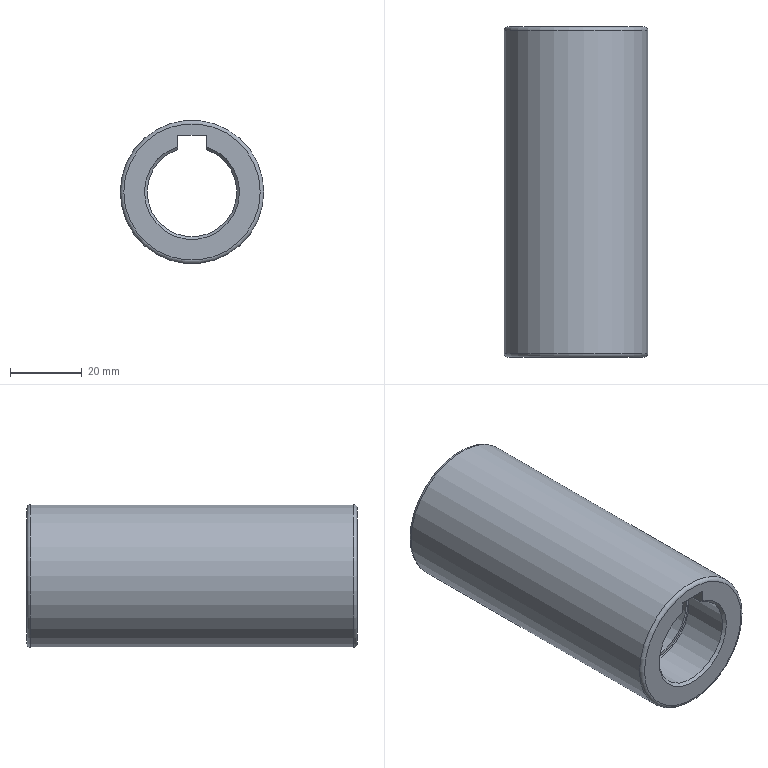Part | STEP file | 冲床-300配套压波_id1126_x_t | 1 solid | 23 faces | box 40 x 92 x 40 mm | volume 67089 mm3 | plane 11 | cylinder 8 | cone 2 | torus 2 | commonest cylinder face diameters 25 x4 26.5 x2 25.5 x1 40 x1
STEP:
#1=CARTESIAN_POINT('',(1388.,32.,91.926));
#2=VERTEX_POINT('',#1);
#3=CARTESIAN_POINT('',(1388.,45.25,91.926));
#4=VERTEX_POINT('',#3);
#5=CARTESIAN_POINT('',(1388.,-46.,91.926));
#6=DIRECTION('',(0.,1.,0.));
#7=VECTOR('',#6,1.);
#8=LINE('',#5,#7);
#9=EDGE_CURVE('',#2,#4,#8,.T.);
#10=ORIENTED_EDGE('',*,*,#9,.T.);
#11=CARTESIAN_POINT('',(1388.,46.,92.715));
#12=VERTEX_POINT('',#11);
#13=CARTESIAN_POINT('',(1388.,45.25,91.926));
#14=CARTESIAN_POINT('',(1388.,45.5,92.19));
#15=CARTESIAN_POINT('',(1388.,45.75,92.453));
#16=CARTESIAN_POINT('',(1388.,46.,92.715));
#17=B_SPLINE_CURVE_WITH_KNOTS('',3,(#13,#14,#15,#16),.UNSPECIFIED.,.F.,.F.,(4,4),(0.,1.),.UNSPECIFIED.);
#18=EDGE_CURVE('',#4,#12,#17,.T.);
#19=ORIENTED_EDGE('',*,*,#18,.T.);
#20=CARTESIAN_POINT('',(1388.,46.,95.883));
#21=VERTEX_POINT('',#20);
#22=CARTESIAN_POINT('',(1388.,46.,95.883));
#23=DIRECTION('',(0.,0.,-1.));
#24=VECTOR('',#23,1.);
#25=LINE('',#22,#24);
#26=EDGE_CURVE('',#21,#12,#25,.T.);
#27=ORIENTED_EDGE('',*,*,#26,.F.);
#28=CARTESIAN_POINT('',(1388.,-46.,95.883));
#29=VERTEX_POINT('',#28);
#30=CARTESIAN_POINT('',(1388.,-46.,95.883));
#31=DIRECTION('',(0.,1.,0.));
#32=VECTOR('',#31,1.);
#33=LINE('',#30,#32);
#34=EDGE_CURVE('',#29,#21,#33,.T.);
#35=ORIENTED_EDGE('',*,*,#34,.F.);
#36=CARTESIAN_POINT('',(1388.,-46.,92.715));
#37=VERTEX_POINT('',#36);
#38=CARTESIAN_POINT('',(1388.,-46.,95.883));
#39=DIRECTION('',(0.,0.,-1.));
#40=VECTOR('',#39,1.);
#41=LINE('',#38,#40);
#42=EDGE_CURVE('',#29,#37,#41,.T.);
#43=ORIENTED_EDGE('',*,*,#42,.T.);
#44=CARTESIAN_POINT('',(1388.,-45.25,91.926));
#45=VERTEX_POINT('',#44);
#46=CARTESIAN_POINT('',(1388.,-46.,92.715));
#47=CARTESIAN_POINT('',(1388.,-45.75,92.453));
#48=CARTESIAN_POINT('',(1388.,-45.5,92.19));
#49=CARTESIAN_POINT('',(1388.,-45.25,91.926));
#50=B_SPLINE_CURVE_WITH_KNOTS('',3,(#46,#47,#48,#49),.UNSPECIFIED.,.F.,.F.,(4,4),(0.,1.),.UNSPECIFIED.);
#51=EDGE_CURVE('',#37,#45,#50,.T.);
#52=ORIENTED_EDGE('',*,*,#51,.T.);
#53=CARTESIAN_POINT('',(1388.,-32.,91.926));
#54=VERTEX_POINT('',#53);
#55=CARTESIAN_POINT('',(1388.,-46.,91.926));
#56=DIRECTION('',(0.,1.,0.));
#57=VECTOR('',#56,1.);
#58=LINE('',#55,#57);
#59=EDGE_CURVE('',#45,#54,#58,.T.);
#60=ORIENTED_EDGE('',*,*,#59,.T.);
#61=CARTESIAN_POINT('',(1388.,-32.,92.715));
#62=VERTEX_POINT('',#61);
#63=CARTESIAN_POINT('',(1388.,-32.,95.883));
#64=DIRECTION('',(0.,0.,1.));
#65=VECTOR('',#64,1.);
#66=LINE('',#63,#65);
#67=EDGE_CURVE('',#54,#62,#66,.T.);
#68=ORIENTED_EDGE('',*,*,#67,.T.);
#69=CARTESIAN_POINT('',(1388.,-31.,92.715));
#70=VERTEX_POINT('',#69);
#71=CARTESIAN_POINT('',(1388.,46.,92.715));
#72=DIRECTION('',(0.,1.,0.));
#73=VECTOR('',#72,1.);
#74=LINE('',#71,#73);
#75=EDGE_CURVE('',#62,#70,#74,.T.);
#76=ORIENTED_EDGE('',*,*,#75,.T.);
#77=CARTESIAN_POINT('',(1388.,-31.,91.926));
#78=VERTEX_POINT('',#77);
#79=CARTESIAN_POINT('',(1388.,-31.,95.883));
#80=DIRECTION('',(0.,0.,-1.));
#81=VECTOR('',#80,1.);
#82=LINE('',#79,#81);
#83=EDGE_CURVE('',#70,#78,#82,.T.);
#84=ORIENTED_EDGE('',*,*,#83,.T.);
#85=CARTESIAN_POINT('',(1388.,-16.,91.926));
#86=VERTEX_POINT('',#85);
#87=CARTESIAN_POINT('',(1388.,-46.,91.926));
#88=DIRECTION('',(0.,1.,0.));
#89=VECTOR('',#88,1.);
#90=LINE('',#87,#89);
#91=EDGE_CURVE('',#78,#86,#90,.T.);
#92=ORIENTED_EDGE('',*,*,#91,.T.);
#93=CARTESIAN_POINT('',(1388.,-16.,92.19));
#94=VERTEX_POINT('',#93);
#95=CARTESIAN_POINT('',(1388.,-16.,95.883));
#96=DIRECTION('',(0.,0.,1.));
#97=VECTOR('',#96,1.);
#98=LINE('',#95,#97);
#99=EDGE_CURVE('',#86,#94,#98,.T.);
#100=ORIENTED_EDGE('',*,*,#99,.T.);
#101=CARTESIAN_POINT('',(1388.,16.,92.19));
#102=VERTEX_POINT('',#101);
#103=CARTESIAN_POINT('',(1388.,46.,92.19));
#104=DIRECTION('',(0.,1.,0.));
#105=VECTOR('',#104,1.);
#106=LINE('',#103,#105);
#107=EDGE_CURVE('',#94,#102,#106,.T.);
#108=ORIENTED_EDGE('',*,*,#107,.T.);
#109=CARTESIAN_POINT('',(1388.,16.,91.926));
#110=VERTEX_POINT('',#109);
#111=CARTESIAN_POINT('',(1388.,16.,95.883));
#112=DIRECTION('',(0.,0.,-1.));
#113=VECTOR('',#112,1.);
#114=LINE('',#111,#113);
#115=EDGE_CURVE('',#102,#110,#114,.T.);
#116=ORIENTED_EDGE('',*,*,#115,.T.);
#117=CARTESIAN_POINT('',(1388.,31.,91.926));
#118=VERTEX_POINT('',#117);
#119=CARTESIAN_POINT('',(1388.,-46.,91.926));
#120=DIRECTION('',(0.,1.,0.));
#121=VECTOR('',#120,1.);
#122=LINE('',#119,#121);
#123=EDGE_CURVE('',#110,#118,#122,.T.);
#124=ORIENTED_EDGE('',*,*,#123,.T.);
#125=CARTESIAN_POINT('',(1388.,31.,92.715));
#126=VERTEX_POINT('',#125);
#127=CARTESIAN_POINT('',(1388.,31.,95.883));
#128=DIRECTION('',(0.,0.,1.));
#129=VECTOR('',#128,1.);
#130=LINE('',#127,#129);
#131=EDGE_CURVE('',#118,#126,#130,.T.);
#132=ORIENTED_EDGE('',*,*,#131,.T.);
#133=CARTESIAN_POINT('',(1388.,32.,92.715));
#134=VERTEX_POINT('',#133);
#135=CARTESIAN_POINT('',(1388.,46.,92.715));
#136=DIRECTION('',(0.,1.,0.));
#137=VECTOR('',#136,1.);
#138=LINE('',#135,#137);
#139=EDGE_CURVE('',#126,#134,#138,.T.);
#140=ORIENTED_EDGE('',*,*,#139,.T.);
#141=CARTESIAN_POINT('',(1388.,32.,95.883));
#142=DIRECTION('',(0.,0.,-1.));
#143=VECTOR('',#142,1.);
#144=LINE('',#141,#143);
#145=EDGE_CURVE('',#134,#2,#144,.T.);
#146=ORIENTED_EDGE('',*,*,#145,.T.);
#147=EDGE_LOOP('',(#10,#19,#27,#35,#43,#52,#60,#68,#76,#84,#92,#100,#108,#116,#124,#132,#140,#146));
#148=FACE_OUTER_BOUND('',#147,.T.);
#149=CARTESIAN_POINT('',(1388.,-46.,95.883));
#150=DIRECTION('',(1.,0.,0.));
#151=DIRECTION('',(0.,0.,-1.));
#152=AXIS2_PLACEMENT_3D('',#149,#150,#151);
#153=PLANE('',#152);
#154=ADVANCED_FACE('',(#148),#153,.T.);
#155=CARTESIAN_POINT('',(1396.,32.,91.926));
#156=VERTEX_POINT('',#155);
#157=CARTESIAN_POINT('',(1396.,45.25,91.926));
#158=VERTEX_POINT('',#157);
#159=CARTESIAN_POINT('',(1396.,-46.,91.926));
#160=DIRECTION('',(0.,1.,0.));
#161=VECTOR('',#160,1.);
#162=LINE('',#159,#161);
#163=EDGE_CURVE('',#156,#158,#162,.T.);
#164=ORIENTED_EDGE('',*,*,#163,.T.);
#165=CARTESIAN_POINT('',(1392.,45.25,80.083));
#166=DIRECTION('',(0.,1.,0.));
#167=DIRECTION('',(1.,0.,0.));
#168=AXIS2_PLACEMENT_3D('',#165,#166,#167);
#169=CIRCLE('',#168,12.5);
#170=EDGE_CURVE('',#158,#4,#169,.T.);
#171=ORIENTED_EDGE('',*,*,#170,.T.);
#172=ORIENTED_EDGE('',*,*,#9,.F.);
#173=CARTESIAN_POINT('',(1392.,32.,80.083));
#174=DIRECTION('',(0.,-1.,0.));
#175=DIRECTION('',(1.,0.,0.));
#176=AXIS2_PLACEMENT_3D('',#173,#174,#175);
#177=CIRCLE('',#176,12.5);
#178=EDGE_CURVE('',#2,#156,#177,.T.);
#179=ORIENTED_EDGE('',*,*,#178,.T.);
#180=EDGE_LOOP('',(#164,#171,#172,#179));
#181=FACE_OUTER_BOUND('',#180,.T.);
#182=CARTESIAN_POINT('',(1392.,-46.,80.083));
#183=DIRECTION('',(0.,1.,0.));
#184=DIRECTION('',(1.,0.,0.));
#185=AXIS2_PLACEMENT_3D('',#182,#183,#184);
#186=CYLINDRICAL_SURFACE('',#185,12.5);
#187=ADVANCED_FACE('',(#181),#186,.F.);
#188=CARTESIAN_POINT('',(1396.,16.,91.926));
#189=VERTEX_POINT('',#188);
#190=CARTESIAN_POINT('',(1396.,31.,91.926));
#191=VERTEX_POINT('',#190);
#192=CARTESIAN_POINT('',(1396.,-46.,91.926));
#193=DIRECTION('',(0.,1.,0.));
#194=VECTOR('',#193,1.);
#195=LINE('',#192,#194);
#196=EDGE_CURVE('',#189,#191,#195,.T.);
#197=ORIENTED_EDGE('',*,*,#196,.T.);
#198=CARTESIAN_POINT('',(1392.,31.,80.083));
#199=DIRECTION('',(0.,1.,0.));
#200=DIRECTION('',(-1.,0.,0.));
#201=AXIS2_PLACEMENT_3D('',#198,#199,#200);
#202=CIRCLE('',#201,12.5);
#203=EDGE_CURVE('',#191,#118,#202,.T.);
#204=ORIENTED_EDGE('',*,*,#203,.T.);
#205=ORIENTED_EDGE('',*,*,#123,.F.);
#206=CARTESIAN_POINT('',(1392.,16.,80.083));
#207=DIRECTION('',(0.,-1.,0.));
#208=DIRECTION('',(1.,0.,0.));
#209=AXIS2_PLACEMENT_3D('',#206,#207,#208);
#210=CIRCLE('',#209,12.5);
#211=EDGE_CURVE('',#110,#189,#210,.T.);
#212=ORIENTED_EDGE('',*,*,#211,.T.);
#213=EDGE_LOOP('',(#197,#204,#205,#212));
#214=FACE_OUTER_BOUND('',#213,.T.);
#215=CARTESIAN_POINT('',(1392.,-46.,80.083));
#216=DIRECTION('',(0.,1.,0.));
#217=DIRECTION('',(1.,0.,0.));
#218=AXIS2_PLACEMENT_3D('',#215,#216,#217);
#219=CYLINDRICAL_SURFACE('',#218,12.5);
#220=ADVANCED_FACE('',(#214),#219,.F.);
#221=ORIENTED_EDGE('',*,*,#59,.F.);
#222=CARTESIAN_POINT('',(1396.,-45.25,91.926));
#223=VERTEX_POINT('',#222);
#224=CARTESIAN_POINT('',(1392.,-45.25,80.083));
#225=DIRECTION('',(0.,-1.,0.));
#226=DIRECTION('',(1.,0.,0.));
#227=AXIS2_PLACEMENT_3D('',#224,#225,#226);
#228=CIRCLE('',#227,12.5);
#229=EDGE_CURVE('',#45,#223,#228,.T.);
#230=ORIENTED_EDGE('',*,*,#229,.T.);
#231=CARTESIAN_POINT('',(1396.,-32.,91.926));
#232=VERTEX_POINT('',#231);
#233=CARTESIAN_POINT('',(1396.,-46.,91.926));
#234=DIRECTION('',(0.,1.,0.));
#235=VECTOR('',#234,1.);
#236=LINE('',#233,#235);
#237=EDGE_CURVE('',#223,#232,#236,.T.);
#238=ORIENTED_EDGE('',*,*,#237,.T.);
#239=CARTESIAN_POINT('',(1392.,-32.,80.083));
#240=DIRECTION('',(0.,1.,0.));
#241=DIRECTION('',(-1.,0.,0.));
#242=AXIS2_PLACEMENT_3D('',#239,#240,#241);
#243=CIRCLE('',#242,12.5);
#244=EDGE_CURVE('',#232,#54,#243,.T.);
#245=ORIENTED_EDGE('',*,*,#244,.T.);
#246=EDGE_LOOP('',(#221,#230,#238,#245));
#247=FACE_OUTER_BOUND('',#246,.T.);
#248=CARTESIAN_POINT('',(1392.,-46.,80.083));
#249=DIRECTION('',(0.,1.,0.));
#250=DIRECTION('',(1.,0.,0.));
#251=AXIS2_PLACEMENT_3D('',#248,#249,#250);
#252=CYLINDRICAL_SURFACE('',#251,12.5);
#253=ADVANCED_FACE('',(#247),#252,.F.);
#254=ORIENTED_EDGE('',*,*,#91,.F.);
#255=CARTESIAN_POINT('',(1396.,-31.,91.926));
#256=VERTEX_POINT('',#255);
#257=CARTESIAN_POINT('',(1392.,-31.,80.083));
#258=DIRECTION('',(0.,-1.,0.));
#259=DIRECTION('',(1.,0.,0.));
#260=AXIS2_PLACEMENT_3D('',#257,#258,#259);
#261=CIRCLE('',#260,12.5);
#262=EDGE_CURVE('',#78,#256,#261,.T.);
#263=ORIENTED_EDGE('',*,*,#262,.T.);
#264=CARTESIAN_POINT('',(1396.,-16.,91.926));
#265=VERTEX_POINT('',#264);
#266=CARTESIAN_POINT('',(1396.,-46.,91.926));
#267=DIRECTION('',(0.,1.,0.));
#268=VECTOR('',#267,1.);
#269=LINE('',#266,#268);
#270=EDGE_CURVE('',#256,#265,#269,.T.);
#271=ORIENTED_EDGE('',*,*,#270,.T.);
#272=CARTESIAN_POINT('',(1392.,-16.,80.083));
#273=DIRECTION('',(0.,1.,0.));
#274=DIRECTION('',(-1.,0.,0.));
#275=AXIS2_PLACEMENT_3D('',#272,#273,#274);
#276=CIRCLE('',#275,12.5);
#277=EDGE_CURVE('',#265,#86,#276,.T.);
#278=ORIENTED_EDGE('',*,*,#277,.T.);
#279=EDGE_LOOP('',(#254,#263,#271,#278));
#280=FACE_OUTER_BOUND('',#279,.T.);
#281=CARTESIAN_POINT('',(1392.,-46.,80.083));
#282=DIRECTION('',(0.,1.,0.));
#283=DIRECTION('',(1.,0.,0.));
#284=AXIS2_PLACEMENT_3D('',#281,#282,#283);
#285=CYLINDRICAL_SURFACE('',#284,12.5);
#286=ADVANCED_FACE('',(#280),#285,.F.);
#287=CARTESIAN_POINT('',(1396.,46.,92.715));
#288=VERTEX_POINT('',#287);
#289=CARTESIAN_POINT('',(1396.,46.,95.883));
#290=VERTEX_POINT('',#289);
#291=CARTESIAN_POINT('',(1396.,46.,95.883));
#292=DIRECTION('',(0.,0.,1.));
#293=VECTOR('',#292,1.);
#294=LINE('',#291,#293);
#295=EDGE_CURVE('',#288,#290,#294,.T.);
#296=ORIENTED_EDGE('',*,*,#295,.F.);
#297=CARTESIAN_POINT('',(1396.,46.,92.715));
#298=CARTESIAN_POINT('',(1396.,45.75,92.453));
#299=CARTESIAN_POINT('',(1396.,45.5,92.19));
#300=CARTESIAN_POINT('',(1396.,45.25,91.926));
#301=B_SPLINE_CURVE_WITH_KNOTS('',3,(#297,#298,#299,#300),.UNSPECIFIED.,.F.,.F.,(4,4),(0.,1.),.UNSPECIFIED.);
#302=EDGE_CURVE('',#288,#158,#301,.T.);
#303=ORIENTED_EDGE('',*,*,#302,.T.);
#304=ORIENTED_EDGE('',*,*,#163,.F.);
#305=CARTESIAN_POINT('',(1396.,32.,92.715));
#306=VERTEX_POINT('',#305);
#307=CARTESIAN_POINT('',(1396.,32.,95.883));
#308=DIRECTION('',(0.,0.,1.));
#309=VECTOR('',#308,1.);
#310=LINE('',#307,#309);
#311=EDGE_CURVE('',#156,#306,#310,.T.);
#312=ORIENTED_EDGE('',*,*,#311,.T.);
#313=CARTESIAN_POINT('',(1396.,31.,92.715));
#314=VERTEX_POINT('',#313);
#315=CARTESIAN_POINT('',(1396.,46.,92.715));
#316=DIRECTION('',(0.,-1.,0.));
#317=VECTOR('',#316,1.);
#318=LINE('',#315,#317);
#319=EDGE_CURVE('',#306,#314,#318,.T.);
#320=ORIENTED_EDGE('',*,*,#319,.T.);
#321=CARTESIAN_POINT('',(1396.,31.,95.883));
#322=DIRECTION('',(0.,0.,-1.));
#323=VECTOR('',#322,1.);
#324=LINE('',#321,#323);
#325=EDGE_CURVE('',#314,#191,#324,.T.);
#326=ORIENTED_EDGE('',*,*,#325,.T.);
#327=ORIENTED_EDGE('',*,*,#196,.F.);
#328=CARTESIAN_POINT('',(1396.,16.,92.19));
#329=VERTEX_POINT('',#328);
#330=CARTESIAN_POINT('',(1396.,16.,95.883));
#331=DIRECTION('',(0.,0.,1.));
#332=VECTOR('',#331,1.);
#333=LINE('',#330,#332);
#334=EDGE_CURVE('',#189,#329,#333,.T.);
#335=ORIENTED_EDGE('',*,*,#334,.T.);
#336=CARTESIAN_POINT('',(1396.,-16.,92.19));
#337=VERTEX_POINT('',#336);
#338=CARTESIAN_POINT('',(1396.,46.,92.19));
#339=DIRECTION('',(0.,-1.,0.));
#340=VECTOR('',#339,1.);
#341=LINE('',#338,#340);
#342=EDGE_CURVE('',#329,#337,#341,.T.);
#343=ORIENTED_EDGE('',*,*,#342,.T.);
#344=CARTESIAN_POINT('',(1396.,-16.,95.883));
#345=DIRECTION('',(0.,0.,-1.));
#346=VECTOR('',#345,1.);
#347=LINE('',#344,#346);
#348=EDGE_CURVE('',#337,#265,#347,.T.);
#349=ORIENTED_EDGE('',*,*,#348,.T.);
#350=ORIENTED_EDGE('',*,*,#270,.F.);
#351=CARTESIAN_POINT('',(1396.,-31.,92.715));
#352=VERTEX_POINT('',#351);
#353=CARTESIAN_POINT('',(1396.,-31.,95.883));
#354=DIRECTION('',(0.,0.,1.));
#355=VECTOR('',#354,1.);
#356=LINE('',#353,#355);
#357=EDGE_CURVE('',#256,#352,#356,.T.);
#358=ORIENTED_EDGE('',*,*,#357,.T.);
#359=CARTESIAN_POINT('',(1396.,-32.,92.715));
#360=VERTEX_POINT('',#359);
#361=CARTESIAN_POINT('',(1396.,46.,92.715));
#362=DIRECTION('',(0.,-1.,0.));
#363=VECTOR('',#362,1.);
#364=LINE('',#361,#363);
#365=EDGE_CURVE('',#352,#360,#364,.T.);
#366=ORIENTED_EDGE('',*,*,#365,.T.);
#367=CARTESIAN_POINT('',(1396.,-32.,95.883));
#368=DIRECTION('',(0.,0.,-1.));
#369=VECTOR('',#368,1.);
#370=LINE('',#367,#369);
#371=EDGE_CURVE('',#360,#232,#370,.T.);
#372=ORIENTED_EDGE('',*,*,#371,.T.);
#373=ORIENTED_EDGE('',*,*,#237,.F.);
#374=CARTESIAN_POINT('',(1396.,-46.,92.715));
#375=VERTEX_POINT('',#374);
#376=CARTESIAN_POINT('',(1396.,-45.25,91.926));
#377=CARTESIAN_POINT('',(1396.,-45.5,92.19));
#378=CARTESIAN_POINT('',(1396.,-45.75,92.453));
#379=CARTESIAN_POINT('',(1396.,-46.,92.715));
#380=B_SPLINE_CURVE_WITH_KNOTS('',3,(#376,#377,#378,#379),.UNSPECIFIED.,.F.,.F.,(4,4),(0.,1.),.UNSPECIFIED.);
#381=EDGE_CURVE('',#223,#375,#380,.T.);
#382=ORIENTED_EDGE('',*,*,#381,.T.);
#383=CARTESIAN_POINT('',(1396.,-46.,95.883));
#384=VERTEX_POINT('',#383);
#385=CARTESIAN_POINT('',(1396.,-46.,95.883));
#386=DIRECTION('',(0.,0.,1.));
#387=VECTOR('',#386,1.);
#388=LINE('',#385,#387);
#389=EDGE_CURVE('',#375,#384,#388,.T.);
#390=ORIENTED_EDGE('',*,*,#389,.T.);
#391=CARTESIAN_POINT('',(1396.,-46.,95.883));
#392=DIRECTION('',(0.,1.,0.));
#393=VECTOR('',#392,1.);
#394=LINE('',#391,#393);
#395=EDGE_CURVE('',#384,#290,#394,.T.);
#396=ORIENTED_EDGE('',*,*,#395,.T.);
#397=EDGE_LOOP('',(#296,#303,#304,#312,#320,#326,#327,#335,#343,#349,#350,#358,#366,#372,#373,#382,#390,#396));
#398=FACE_OUTER_BOUND('',#397,.T.);
#399=CARTESIAN_POINT('',(1396.,-46.,95.883));
#400=DIRECTION('',(-1.,0.,0.));
#401=DIRECTION('',(0.,0.,1.));
#402=AXIS2_PLACEMENT_3D('',#399,#400,#401);
#403=PLANE('',#402);
#404=ADVANCED_FACE('',(#398),#403,.T.);
#405=CARTESIAN_POINT('',(1411.,-46.,80.083));
#406=VERTEX_POINT('',#405);
#407=CARTESIAN_POINT('',(1392.,-46.,80.083));
#408=DIRECTION('',(0.,-1.,0.));
#409=DIRECTION('',(1.,0.,0.));
#410=AXIS2_PLACEMENT_3D('',#407,#408,#409);
#411=CIRCLE('',#410,19.);
#412=EDGE_CURVE('',#406,#406,#411,.T.);
#413=ORIENTED_EDGE('',*,*,#412,.T.);
#414=EDGE_LOOP('',(#413));
#415=FACE_BOUND('',#414,.T.);
#416=ORIENTED_EDGE('',*,*,#389,.F.);
#417=CARTESIAN_POINT('',(1392.,-46.,80.083));
#418=DIRECTION('',(0.,1.,0.));
#419=DIRECTION('',(1.,0.,0.));
#420=AXIS2_PLACEMENT_3D('',#417,#418,#419);
#421=CIRCLE('',#420,13.25);
#422=EDGE_CURVE('',#375,#37,#421,.T.);
#423=ORIENTED_EDGE('',*,*,#422,.T.);
#424=ORIENTED_EDGE('',*,*,#42,.F.);
#425=CARTESIAN_POINT('',(1388.,-46.,95.883));
#426=DIRECTION('',(-1.,0.,0.));
#427=VECTOR('',#426,1.);
#428=LINE('',#425,#427);
#429=EDGE_CURVE('',#384,#29,#428,.T.);
#430=ORIENTED_EDGE('',*,*,#429,.F.);
#431=EDGE_LOOP('',(#416,#423,#424,#430));
#432=FACE_BOUND('',#431,.T.);
#433=CARTESIAN_POINT('',(1392.,-46.,80.083));
#434=DIRECTION('',(0.,-1.,0.));
#435=DIRECTION('',(-1.,0.,0.));
#436=AXIS2_PLACEMENT_3D('',#433,#434,#435);
#437=PLANE('',#436);
#438=ADVANCED_FACE('',(#415,#432),#437,.T.);
#439=CARTESIAN_POINT('',(1411.,46.,80.083));
#440=VERTEX_POINT('',#439);
#441=CARTESIAN_POINT('',(1392.,46.,80.083));
#442=DIRECTION('',(0.,1.,0.));
#443=DIRECTION('',(1.,0.,0.));
#444=AXIS2_PLACEMENT_3D('',#441,#442,#443);
#445=CIRCLE('',#444,19.);
#446=EDGE_CURVE('',#440,#440,#445,.T.);
#447=ORIENTED_EDGE('',*,*,#446,.T.);
#448=EDGE_LOOP('',(#447));
#449=FACE_BOUND('',#448,.T.);
#450=ORIENTED_EDGE('',*,*,#26,.T.);
#451=CARTESIAN_POINT('',(1392.,46.,80.083));
#452=DIRECTION('',(0.,-1.,0.));
#453=DIRECTION('',(1.,0.,0.));
#454=AXIS2_PLACEMENT_3D('',#451,#452,#453);
#455=CIRCLE('',#454,13.25);
#456=EDGE_CURVE('',#12,#288,#455,.T.);
#457=ORIENTED_EDGE('',*,*,#456,.T.);
#458=ORIENTED_EDGE('',*,*,#295,.T.);
#459=CARTESIAN_POINT('',(1388.,46.,95.883));
#460=DIRECTION('',(-1.,0.,0.));
#461=VECTOR('',#460,1.);
#462=LINE('',#459,#461);
#463=EDGE_CURVE('',#290,#21,#462,.T.);
#464=ORIENTED_EDGE('',*,*,#463,.T.);
#465=EDGE_LOOP('',(#450,#457,#458,#464));
#466=FACE_BOUND('',#465,.T.);
#467=CARTESIAN_POINT('',(1392.,46.,80.083));
#468=DIRECTION('',(0.,-1.,0.));
#469=DIRECTION('',(-1.,0.,0.));
#470=AXIS2_PLACEMENT_3D('',#467,#468,#469);
#471=PLANE('',#470);
#472=ADVANCED_FACE('',(#449,#466),#471,.F.);
#473=CARTESIAN_POINT('',(1412.,45.,80.083));
#474=VERTEX_POINT('',#473);
#475=CARTESIAN_POINT('',(1392.,45.,80.083));
#476=DIRECTION('',(0.,-1.,0.));
#477=DIRECTION('',(1.,0.,0.));
#478=AXIS2_PLACEMENT_3D('',#475,#476,#477);
#479=CIRCLE('',#478,20.);
#480=EDGE_CURVE('',#474,#474,#479,.T.);
#481=ORIENTED_EDGE('',*,*,#480,.T.);
#482=EDGE_LOOP('',(#481));
#483=FACE_BOUND('',#482,.T.);
#484=CARTESIAN_POINT('',(1412.,-45.,80.083));
#485=VERTEX_POINT('',#484);
#486=CARTESIAN_POINT('',(1392.,-45.,80.083));
#487=DIRECTION('',(0.,1.,0.));
#488=DIRECTION('',(1.,0.,0.));
#489=AXIS2_PLACEMENT_3D('',#486,#487,#488);
#490=CIRCLE('',#489,20.);
#491=EDGE_CURVE('',#485,#485,#490,.T.);
#492=ORIENTED_EDGE('',*,*,#491,.T.);
#493=EDGE_LOOP('',(#492));
#494=FACE_BOUND('',#493,.T.);
#495=CARTESIAN_POINT('',(1392.,-46.,80.083));
#496=DIRECTION('',(0.,1.,0.));
#497=DIRECTION('',(1.,0.,0.));
#498=AXIS2_PLACEMENT_3D('',#495,#496,#497);
#499=CYLINDRICAL_SURFACE('',#498,20.);
#500=ADVANCED_FACE('',(#483,#494),#499,.T.);
#501=ORIENTED_EDGE('',*,*,#463,.F.);
#502=ORIENTED_EDGE('',*,*,#395,.F.);
#503=ORIENTED_EDGE('',*,*,#429,.T.);
#504=ORIENTED_EDGE('',*,*,#34,.T.);
#505=EDGE_LOOP('',(#501,#502,#503,#504));
#506=FACE_OUTER_BOUND('',#505,.T.);
#507=CARTESIAN_POINT('',(1388.,-46.,95.883));
#508=DIRECTION('',(0.,0.,-1.));
#509=DIRECTION('',(-1.,0.,0.));
#510=AXIS2_PLACEMENT_3D('',#507,#508,#509);
#511=PLANE('',#510);
#512=ADVANCED_FACE('',(#506),#511,.T.);
#513=CARTESIAN_POINT('',(1392.,16.,80.083));
#514=DIRECTION('',(0.,1.,0.));
#515=DIRECTION('',(-1.,0.,0.));
#516=AXIS2_PLACEMENT_3D('',#513,#514,#515);
#517=CIRCLE('',#516,12.75);
#518=EDGE_CURVE('',#329,#102,#517,.T.);
#519=ORIENTED_EDGE('',*,*,#518,.F.);
#520=ORIENTED_EDGE('',*,*,#334,.F.);
#521=ORIENTED_EDGE('',*,*,#211,.F.);
#522=ORIENTED_EDGE('',*,*,#115,.F.);
#523=EDGE_LOOP('',(#519,#520,#521,#522));
#524=FACE_OUTER_BOUND('',#523,.T.);
#525=CARTESIAN_POINT('',(1392.,16.,92.833));
#526=DIRECTION('',(0.,-1.,0.));
#527=DIRECTION('',(-1.,0.,0.));
#528=AXIS2_PLACEMENT_3D('',#525,#526,#527);
#529=PLANE('',#528);
#530=ADVANCED_FACE('',(#524),#529,.T.);
#531=ORIENTED_EDGE('',*,*,#277,.F.);
#532=ORIENTED_EDGE('',*,*,#348,.F.);
#533=CARTESIAN_POINT('',(1392.,-16.,80.083));
#534=DIRECTION('',(0.,1.,0.));
#535=DIRECTION('',(-1.,0.,0.));
#536=AXIS2_PLACEMENT_3D('',#533,#534,#535);
#537=CIRCLE('',#536,12.75);
#538=EDGE_CURVE('',#337,#94,#537,.T.);
#539=ORIENTED_EDGE('',*,*,#538,.T.);
#540=ORIENTED_EDGE('',*,*,#99,.F.);
#541=EDGE_LOOP('',(#531,#532,#539,#540));
#542=FACE_OUTER_BOUND('',#541,.T.);
#543=CARTESIAN_POINT('',(1392.,-16.,92.833));
#544=DIRECTION('',(0.,1.,0.));
#545=DIRECTION('',(1.,0.,0.));
#546=AXIS2_PLACEMENT_3D('',#543,#544,#545);
#547=PLANE('',#546);
#548=ADVANCED_FACE('',(#542),#547,.T.);
#549=ORIENTED_EDGE('',*,*,#538,.F.);
#550=ORIENTED_EDGE('',*,*,#342,.F.);
#551=ORIENTED_EDGE('',*,*,#518,.T.);
#552=ORIENTED_EDGE('',*,*,#107,.F.);
#553=EDGE_LOOP('',(#549,#550,#551,#552));
#554=FACE_OUTER_BOUND('',#553,.T.);
#555=CARTESIAN_POINT('',(1392.,46.,80.083));
#556=DIRECTION('',(0.,1.,0.));
#557=DIRECTION('',(1.,0.,0.));
#558=AXIS2_PLACEMENT_3D('',#555,#556,#557);
#559=CYLINDRICAL_SURFACE('',#558,12.75);
#560=ADVANCED_FACE('',(#554),#559,.F.);
#561=CARTESIAN_POINT('',(1392.,31.,80.083));
#562=DIRECTION('',(0.,1.,0.));
#563=DIRECTION('',(-1.,0.,0.));
#564=AXIS2_PLACEMENT_3D('',#561,#562,#563);
#565=CIRCLE('',#564,13.25);
#566=EDGE_CURVE('',#314,#126,#565,.T.);
#567=ORIENTED_EDGE('',*,*,#566,.F.);
#568=ORIENTED_EDGE('',*,*,#319,.F.);
#569=CARTESIAN_POINT('',(1392.,32.,80.083));
#570=DIRECTION('',(0.,1.,0.));
#571=DIRECTION('',(-1.,0.,0.));
#572=AXIS2_PLACEMENT_3D('',#569,#570,#571);
#573=CIRCLE('',#572,13.25);
#574=EDGE_CURVE('',#306,#134,#573,.T.);
#575=ORIENTED_EDGE('',*,*,#574,.T.);
#576=ORIENTED_EDGE('',*,*,#139,.F.);
#577=EDGE_LOOP('',(#567,#568,#575,#576));
#578=FACE_OUTER_BOUND('',#577,.T.);
#579=CARTESIAN_POINT('',(1392.,46.,80.083));
#580=DIRECTION('',(0.,1.,0.));
#581=DIRECTION('',(1.,0.,0.));
#582=AXIS2_PLACEMENT_3D('',#579,#580,#581);
#583=CYLINDRICAL_SURFACE('',#582,13.25);
#584=ADVANCED_FACE('',(#578),#583,.F.);
#585=ORIENTED_EDGE('',*,*,#574,.F.);
#586=ORIENTED_EDGE('',*,*,#311,.F.);
#587=ORIENTED_EDGE('',*,*,#178,.F.);
#588=ORIENTED_EDGE('',*,*,#145,.F.);
#589=EDGE_LOOP('',(#585,#586,#587,#588));
#590=FACE_OUTER_BOUND('',#589,.T.);
#591=CARTESIAN_POINT('',(1392.,32.,80.083));
#592=DIRECTION('',(0.,-1.,0.));
#593=DIRECTION('',(-1.,0.,0.));
#594=AXIS2_PLACEMENT_3D('',#591,#592,#593);
#595=PLANE('',#594);
#596=ADVANCED_FACE('',(#590),#595,.T.);
#597=ORIENTED_EDGE('',*,*,#203,.F.);
#598=ORIENTED_EDGE('',*,*,#325,.F.);
#599=ORIENTED_EDGE('',*,*,#566,.T.);
#600=ORIENTED_EDGE('',*,*,#131,.F.);
#601=EDGE_LOOP('',(#597,#598,#599,#600));
#602=FACE_OUTER_BOUND('',#601,.T.);
#603=CARTESIAN_POINT('',(1392.,31.,80.083));
#604=DIRECTION('',(0.,1.,0.));
#605=DIRECTION('',(1.,0.,0.));
#606=AXIS2_PLACEMENT_3D('',#603,#604,#605);
#607=PLANE('',#606);
#608=ADVANCED_FACE('',(#602),#607,.T.);
#609=CARTESIAN_POINT('',(1392.,-32.,80.083));
#610=DIRECTION('',(0.,1.,0.));
#611=DIRECTION('',(-1.,0.,0.));
#612=AXIS2_PLACEMENT_3D('',#609,#610,#611);
#613=CIRCLE('',#612,13.25);
#614=EDGE_CURVE('',#360,#62,#613,.T.);
#615=ORIENTED_EDGE('',*,*,#614,.F.);
#616=ORIENTED_EDGE('',*,*,#365,.F.);
#617=CARTESIAN_POINT('',(1392.,-31.,80.083));
#618=DIRECTION('',(0.,1.,0.));
#619=DIRECTION('',(-1.,0.,0.));
#620=AXIS2_PLACEMENT_3D('',#617,#618,#619);
#621=CIRCLE('',#620,13.25);
#622=EDGE_CURVE('',#352,#70,#621,.T.);
#623=ORIENTED_EDGE('',*,*,#622,.T.);
#624=ORIENTED_EDGE('',*,*,#75,.F.);
#625=EDGE_LOOP('',(#615,#616,#623,#624));
#626=FACE_OUTER_BOUND('',#625,.T.);
#627=CARTESIAN_POINT('',(1392.,46.,80.083));
#628=DIRECTION('',(0.,1.,0.));
#629=DIRECTION('',(1.,0.,0.));
#630=AXIS2_PLACEMENT_3D('',#627,#628,#629);
#631=CYLINDRICAL_SURFACE('',#630,13.25);
#632=ADVANCED_FACE('',(#626),#631,.F.);
#633=ORIENTED_EDGE('',*,*,#244,.F.);
#634=ORIENTED_EDGE('',*,*,#371,.F.);
#635=ORIENTED_EDGE('',*,*,#614,.T.);
#636=ORIENTED_EDGE('',*,*,#67,.F.);
#637=EDGE_LOOP('',(#633,#634,#635,#636));
#638=FACE_OUTER_BOUND('',#637,.T.);
#639=CARTESIAN_POINT('',(1392.,-32.,80.083));
#640=DIRECTION('',(0.,1.,0.));
#641=DIRECTION('',(1.,0.,0.));
#642=AXIS2_PLACEMENT_3D('',#639,#640,#641);
#643=PLANE('',#642);
#644=ADVANCED_FACE('',(#638),#643,.T.);
#645=ORIENTED_EDGE('',*,*,#622,.F.);
#646=ORIENTED_EDGE('',*,*,#357,.F.);
#647=ORIENTED_EDGE('',*,*,#262,.F.);
#648=ORIENTED_EDGE('',*,*,#83,.F.);
#649=EDGE_LOOP('',(#645,#646,#647,#648));
#650=FACE_OUTER_BOUND('',#649,.T.);
#651=CARTESIAN_POINT('',(1392.,-31.,80.083));
#652=DIRECTION('',(0.,-1.,0.));
#653=DIRECTION('',(-1.,0.,0.));
#654=AXIS2_PLACEMENT_3D('',#651,#652,#653);
#655=PLANE('',#654);
#656=ADVANCED_FACE('',(#650),#655,.T.);
#657=ORIENTED_EDGE('',*,*,#18,.F.);
#658=ORIENTED_EDGE('',*,*,#170,.F.);
#659=ORIENTED_EDGE('',*,*,#302,.F.);
#660=ORIENTED_EDGE('',*,*,#456,.F.);
#661=EDGE_LOOP('',(#657,#658,#659,#660));
#662=FACE_OUTER_BOUND('',#661,.T.);
#663=CARTESIAN_POINT('',(1392.,46.,80.083));
#664=DIRECTION('',(0.,1.,0.));
#665=DIRECTION('',(1.,0.,0.));
#666=AXIS2_PLACEMENT_3D('',#663,#664,#665);
#667=CONICAL_SURFACE('',#666,13.25,45.);
#668=ADVANCED_FACE('',(#662),#667,.F.);
#669=ORIENTED_EDGE('',*,*,#51,.F.);
#670=ORIENTED_EDGE('',*,*,#422,.F.);
#671=ORIENTED_EDGE('',*,*,#381,.F.);
#672=ORIENTED_EDGE('',*,*,#229,.F.);
#673=EDGE_LOOP('',(#669,#670,#671,#672));
#674=FACE_OUTER_BOUND('',#673,.T.);
#675=CARTESIAN_POINT('',(1392.,-45.25,80.083));
#676=DIRECTION('',(0.,-1.,0.));
#677=DIRECTION('',(-1.,0.,0.));
#678=AXIS2_PLACEMENT_3D('',#675,#676,#677);
#679=CONICAL_SURFACE('',#678,12.5,45.);
#680=ADVANCED_FACE('',(#674),#679,.F.);
#681=ORIENTED_EDGE('',*,*,#480,.F.);
#682=EDGE_LOOP('',(#681));
#683=FACE_BOUND('',#682,.T.);
#684=ORIENTED_EDGE('',*,*,#446,.F.);
#685=EDGE_LOOP('',(#684));
#686=FACE_BOUND('',#685,.T.);
#687=CARTESIAN_POINT('',(1392.,45.,80.083));
#688=DIRECTION('',(0.,-1.,0.));
#689=DIRECTION('',(-1.,0.,0.));
#690=AXIS2_PLACEMENT_3D('',#687,#688,#689);
#691=TOROIDAL_SURFACE('',#690,19.,1.);
#692=ADVANCED_FACE('',(#683,#686),#691,.T.);
#693=ORIENTED_EDGE('',*,*,#412,.F.);
#694=EDGE_LOOP('',(#693));
#695=FACE_BOUND('',#694,.T.);
#696=ORIENTED_EDGE('',*,*,#491,.F.);
#697=EDGE_LOOP('',(#696));
#698=FACE_BOUND('',#697,.T.);
#699=CARTESIAN_POINT('',(1392.,-45.,80.083));
#700=DIRECTION('',(0.,-1.,0.));
#701=DIRECTION('',(-1.,0.,0.));
#702=AXIS2_PLACEMENT_3D('',#699,#700,#701);
#703=TOROIDAL_SURFACE('',#702,19.,1.);
#704=ADVANCED_FACE('',(#695,#698),#703,.T.);
#705=CLOSED_SHELL('',(#154,#187,#220,#253,#286,#404,#438,#472,#500,#512,#530,#548,#560,#584,#596,#608,#632,#644,#656,#668,#680,#692,#704));
#706=MANIFOLD_SOLID_BREP('',#705);
#707=(LENGTH_UNIT()NAMED_UNIT(*)SI_UNIT(.MILLI.,.METRE.));
#708=UNCERTAINTY_MEASURE_WITH_UNIT(LENGTH_MEASURE(0.00002),#707,'','');
#709=(NAMED_UNIT(*)PLANE_ANGLE_UNIT()SI_UNIT($,.RADIAN.));
#710=PLANE_ANGLE_MEASURE_WITH_UNIT(PLANE_ANGLE_MEASURE(0.01745),#709);
#711=DIMENSIONAL_EXPONENTS(0.,0.,0.,0.,0.,0.,0.);
#712=(CONVERSION_BASED_UNIT('DEGREE',#710)NAMED_UNIT(#711)PLANE_ANGLE_UNIT());
#713=(NAMED_UNIT(*)SI_UNIT($,.STERADIAN.)SOLID_ANGLE_UNIT());
#714=(GEOMETRIC_REPRESENTATION_CONTEXT(3)GLOBAL_UNCERTAINTY_ASSIGNED_CONTEXT((#708))GLOBAL_UNIT_ASSIGNED_CONTEXT((#707,#712,#713))REPRESENTATION_CONTEXT('',''));
#715=ADVANCED_BREP_SHAPE_REPRESENTATION('',(#706),#714);